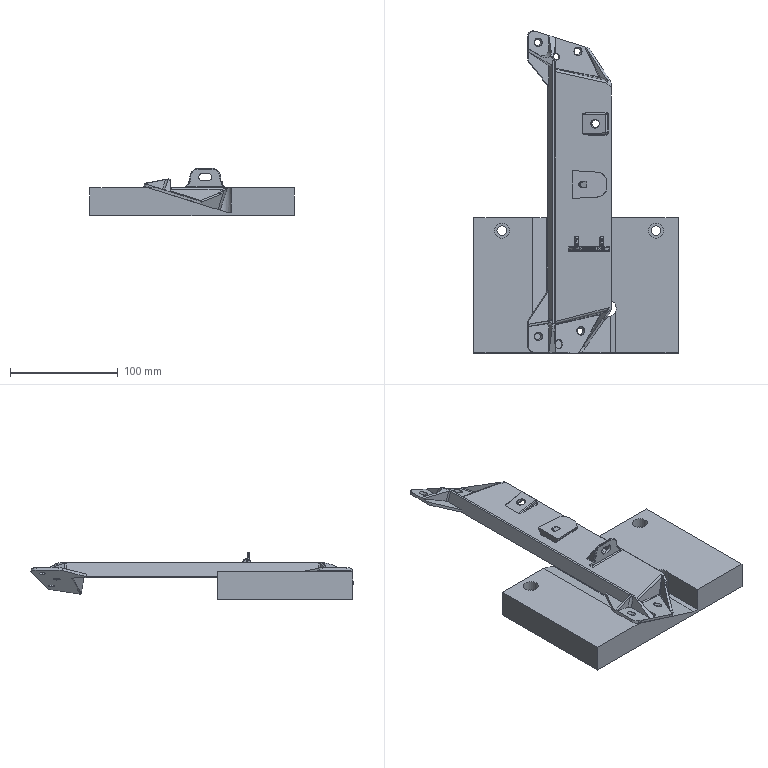NC program | NX | posted with a generic post | part box 190 x 299.709 x 43.804 mm
Whole program:
N10 G17 G21 G94 G90
(PLANAR_MILL_4_COPY_COPY_2_COPY_COPY_1_COPY , TOOL : D4)
N12 T03 M6
N14 G53
N16 G17 G0 G90 X-12.473 Y-11.4 S5800 M3
N18 G43 Z10. H3
N20 Z-95.192
N22 G94 G1 X-9.816 Z-95.206 F2500.
N24 X-9.648 Z-95.207
N26 X-9.199 Y-11.268 Z-95.209
N28 X-8.818 Y-10.997 Z-95.212
N30 X-8.547 Y-10.616 Z-95.214
N32 X-8.416 Y-10.167 Z-95.217
N34 Y-9.832 Z-95.218
N36 X-8.548 Y-9.383 Z-95.221
N38 X-8.819 Y-9.002 Z-95.223
N40 X-9.2 Y-8.731 Z-95.226
N42 X-9.649 Y-8.6 Z-95.228
N44 X-14.987 Z-95.256
N46 X-15.435 Y-8.732 Z-95.258
N48 X-15.816 Y-9.003 Z-95.261
N50 X-16.087 Y-9.384 Z-95.263
N52 X-16.219 Y-9.833 Z-95.266
N54 Y-10.168 Z-95.268
N56 X-16.087 Y-10.617 Z-95.27
N58 X-15.816 Y-10.997 Z-95.272
N60 X-15.435 Y-11.268 Z-95.275
N62 X-14.986 Y-11.4 Z-95.277
N64 X-9.648 Z-95.305
N66 X-9.199 Y-11.268 Z-95.308
N68 X-8.818 Y-10.997 Z-95.31
N70 X-8.547 Y-10.616 Z-95.313
N72 X-8.416 Y-10.167 Z-95.315
N74 Y-9.832 Z-95.317
N76 X-8.548 Y-9.383 Z-95.319
N78 X-8.819 Y-9.002 Z-95.322
N80 X-9.2 Y-8.731 Z-95.324
N82 X-9.649 Y-8.6 Z-95.327
N84 X-14.987 Z-95.355
N86 X-15.435 Y-8.732 Z-95.357
N88 X-15.816 Y-9.003 Z-95.36
N90 X-16.087 Y-9.384 Z-95.362
N92 X-16.219 Y-9.833 Z-95.364
N94 Y-10.168 Z-95.366
N96 X-16.087 Y-10.617 Z-95.369
N98 X-15.816 Y-10.997 Z-95.371
N100 X-15.435 Y-11.268 Z-95.374
N102 X-14.986 Y-11.4 Z-95.376
N104 X-9.648 Z-95.404
N106 X-9.199 Y-11.268 Z-95.406
N108 X-8.818 Y-10.997 Z-95.409
N110 X-8.547 Y-10.616 Z-95.411
N112 X-8.416 Y-10.167 Z-95.414
N114 Y-9.832 Z-95.415
N116 X-8.548 Y-9.383 Z-95.418
N118 X-8.819 Y-9.002 Z-95.42
N120 X-9.2 Y-8.731 Z-95.423
N122 X-9.649 Y-8.6 Z-95.425
N124 X-14.987 Z-95.453
N126 X-15.435 Y-8.732 Z-95.456
N128 X-15.816 Y-9.003 Z-95.458
N130 X-16.087 Y-9.384 Z-95.461
N132 X-16.219 Y-9.833 Z-95.463
N134 Y-10.168 Z-95.465
N136 X-16.087 Y-10.617 Z-95.467
N138 X-15.816 Y-10.997 Z-95.47
N140 X-15.435 Y-11.268 Z-95.472
N142 X-14.986 Y-11.4 Z-95.475
N144 X-9.648 Z-95.502
N146 X-9.199 Y-11.268 Z-95.505
N148 X-8.818 Y-10.997 Z-95.507
N150 X-8.547 Y-10.616 Z-95.51
N152 X-8.416 Y-10.167 Z-95.512
N154 Y-9.832 Z-95.514
N156 X-8.548 Y-9.383 Z-95.516
N158 X-8.819 Y-9.002 Z-95.519
N160 X-9.2 Y-8.731 Z-95.521
N162 X-9.649 Y-8.6 Z-95.524
N164 X-14.987 Z-95.552
N166 X-15.435 Y-8.732 Z-95.554
N168 X-15.816 Y-9.003 Z-95.557
N170 X-16.087 Y-9.384 Z-95.559
N172 X-16.219 Y-9.833 Z-95.562
N174 Y-10.168 Z-95.563
N176 X-16.087 Y-10.617 Z-95.566
N178 X-15.816 Y-10.997 Z-95.568
N180 X-15.435 Y-11.268 Z-95.571
N182 X-14.986 Y-11.4 Z-95.573
N184 X-9.648 Z-95.601
N186 X-9.199 Y-11.268 Z-95.604
N188 X-8.818 Y-10.997 Z-95.606
N190 X-8.547 Y-10.616 Z-95.608
N192 X-8.416 Y-10.167 Z-95.611
N194 Y-9.832 Z-95.613
N196 X-8.548 Y-9.383 Z-95.615
N198 X-8.819 Y-9.002 Z-95.618
N200 X-9.2 Y-8.731 Z-95.62
N202 X-9.649 Y-8.6 Z-95.622
N204 X-14.987 Z-95.65
N206 X-15.435 Y-8.732 Z-95.653
N208 X-15.816 Y-9.003 Z-95.655
N210 X-16.087 Y-9.384 Z-95.658
N212 X-16.219 Y-9.833 Z-95.66
N214 Y-10.168 Z-95.662
N216 X-16.087 Y-10.617 Z-95.664
N218 X-15.816 Y-10.997 Z-95.667
N220 X-15.435 Y-11.268 Z-95.669
N222 X-14.986 Y-11.4 Z-95.672
N224 X-9.648 Z-95.7
N226 X-9.199 Y-11.268 Z-95.702
N228 X-8.818 Y-10.997 Z-95.705
N230 X-8.547 Y-10.616 Z-95.707
N232 X-8.416 Y-10.167 Z-95.709
N234 Y-9.832 Z-95.711
N236 X-8.548 Y-9.383 Z-95.714
N238 X-8.819 Y-9.002 Z-95.716
N240 X-9.2 Y-8.731 Z-95.719
N242 X-9.649 Y-8.6 Z-95.721
N244 X-14.987 Z-95.749
N246 X-15.435 Y-8.732 Z-95.751
N248 X-15.816 Y-9.003 Z-95.754
N250 X-16.087 Y-9.384 Z-95.756
N252 X-16.219 Y-9.833 Z-95.759
N254 Y-10.168 Z-95.76
N256 X-16.087 Y-10.617 Z-95.763
N258 X-15.816 Y-10.997 Z-95.765
N260 X-15.435 Y-11.268 Z-95.768
N262 X-14.986 Y-11.4 Z-95.77
N264 X-9.648 Z-95.798
N266 X-9.199 Y-11.268 Z-95.801
N268 X-8.818 Y-10.997 Z-95.803
N270 X-8.547 Y-10.616 Z-95.806
N272 X-8.416 Y-10.167 Z-95.808
N274 Y-9.832 Z-95.81
N276 X-8.548 Y-9.383 Z-95.812
N278 X-8.819 Y-9.002 Z-95.815
N280 X-9.2 Y-8.731 Z-95.817
N282 X-9.649 Y-8.6 Z-95.82
N284 X-14.987 Z-95.848
N286 X-15.435 Y-8.732 Z-95.85
N288 X-15.816 Y-9.003 Z-95.852
N290 X-16.087 Y-9.384 Z-95.855
N292 X-16.219 Y-9.833 Z-95.857
N294 Y-10.168 Z-95.859
N296 X-16.087 Y-10.617 Z-95.862
N298 X-15.816 Y-10.997 Z-95.864
N300 X-15.435 Y-11.268 Z-95.866
N302 X-14.986 Y-11.4 Z-95.869
N304 X-9.648 Z-95.897
N306 X-9.199 Y-11.268 Z-95.899
N308 X-8.818 Y-10.997 Z-95.902
N310 X-8.547 Y-10.616 Z-95.904
N312 X-8.416 Y-10.167 Z-95.907
N314 Y-9.832 Z-95.908
N316 X-8.548 Y-9.383 Z-95.911
N318 X-8.819 Y-9.002 Z-95.913
N320 X-9.2 Y-8.731 Z-95.916
N322 X-9.649 Y-8.6 Z-95.918
N324 X-14.987 Z-95.946
N326 X-15.435 Y-8.732 Z-95.949
N328 X-15.816 Y-9.003 Z-95.951
N330 X-16.087 Y-9.384 Z-95.953
N332 X-16.219 Y-9.833 Z-95.956
N334 Y-10.168 Z-95.958
N336 X-16.087 Y-10.617 Z-95.96
N338 X-15.816 Y-10.997 Z-95.963
N340 X-15.435 Y-11.268 Z-95.965
N342 X-14.986 Y-11.4 Z-95.967
N344 X-9.648 Z-95.995
N346 X-9.199 Y-11.268 Z-95.998
N348 X-8.818 Y-10.997 Z-96.
N350 X-8.547 Y-10.616 Z-96.003
N352 X-8.416 Y-10.167 Z-96.005
N354 Y-9.832 Z-96.007
N356 X-8.548 Y-9.383 Z-96.009
N358 X-8.819 Y-9.002 Z-96.012
N360 X-9.2 Y-8.731 Z-96.014
N362 X-9.649 Y-8.6 Z-96.017
N364 X-14.987 Z-96.045
N366 X-15.435 Y-8.732 Z-96.047
N368 X-15.816 Y-9.003 Z-96.05
N370 X-16.087 Y-9.384 Z-96.052
N372 X-16.219 Y-9.833 Z-96.054
N374 Y-10.168 Z-96.056
N376 X-16.087 Y-10.617 Z-96.059
N378 X-15.816 Y-10.997 Z-96.061
N380 X-15.435 Y-11.268 Z-96.064
N382 X-14.986 Y-11.4 Z-96.066
N384 X-9.648 Z-96.094
N386 X-9.199 Y-11.268 Z-96.096
N388 X-8.818 Y-10.997 Z-96.099
N390 X-8.547 Y-10.616 Z-96.101
N392 X-8.416 Y-10.167 Z-96.104
N394 Y-9.832 Z-96.106
N396 X-8.548 Y-9.383 Z-96.108
N398 X-8.819 Y-9.002 Z-96.11
N400 X-9.2 Y-8.731 Z-96.113
N402 X-9.649 Y-8.6 Z-96.115
N404 X-14.987 Z-96.143
N406 X-15.435 Y-8.732 Z-96.146
N408 X-15.816 Y-9.003 Z-96.148
N410 X-16.087 Y-9.384 Z-96.151
N412 X-16.219 Y-9.833 Z-96.153
N414 Y-10.168 Z-96.155
N416 X-16.087 Y-10.617 Z-96.157
N418 X-15.816 Y-10.997 Z-96.16
N420 X-15.435 Y-11.268 Z-96.162
N422 X-14.986 Y-11.4 Z-96.165
N424 X-9.648 Z-96.193
N426 X-9.199 Y-11.268 Z-96.195
N428 X-8.818 Y-10.997 Z-96.197
N430 X-8.547 Y-10.616 Z-96.2
N432 X-8.416 Y-10.167 Z-96.202
N434 Y-9.832 Z-96.204
N436 X-8.548 Y-9.383 Z-96.207
N438 X-8.819 Y-9.002 Z-96.209
N440 X-9.2 Y-8.731 Z-96.211
N442 X-9.649 Y-8.6 Z-96.214
N444 X-14.987 Z-96.242
N446 X-15.435 Y-8.732 Z-96.244
N448 X-15.816 Y-9.003 Z-96.247
N450 X-16.087 Y-9.384 Z-96.249
N452 X-16.219 Y-9.833 Z-96.252
N454 Y-10.168 Z-96.253
N456 X-16.087 Y-10.617 Z-96.256
N458 X-15.816 Y-10.997 Z-96.258
N460 X-15.435 Y-11.268 Z-96.261
N462 X-14.986 Y-11.4 Z-96.263
N464 X-9.648 Z-96.291
N466 X-9.199 Y-11.268 Z-96.294
N468 X-8.818 Y-10.997 Z-96.296
N470 X-8.547 Y-10.616 Z-96.299
N472 X-8.416 Y-10.167 Z-96.301
N474 Y-9.832 Z-96.303
N476 X-8.548 Y-9.383 Z-96.305
N478 X-8.819 Y-9.002 Z-96.308
N480 X-9.2 Y-8.731 Z-96.31
N482 X-9.649 Y-8.6 Z-96.312
N484 X-14.987 Z-96.34
N486 X-15.435 Y-8.732 Z-96.343
N488 X-15.816 Y-9.003 Z-96.345
N490 X-16.087 Y-9.384 Z-96.348
N492 X-16.219 Y-9.833 Z-96.35
N494 Y-10.168 Z-96.352
N496 X-16.087 Y-10.617 Z-96.354
N498 X-15.816 Y-10.997 Z-96.357
N500 X-15.435 Y-11.268 Z-96.359
N502 X-14.986 Y-11.4 Z-96.362
N504 X-9.648 Z-96.39
N506 X-9.199 Y-11.268 Z-96.392
N508 X-8.818 Y-10.997 Z-96.395
N510 X-8.547 Y-10.616 Z-96.397
N512 X-8.416 Y-10.167 Z-96.4
N514 Y-9.832 Z-96.401
N516 X-8.548 Y-9.383 Z-96.404
N518 X-8.819 Y-9.002 Z-96.406
N520 X-9.2 Y-8.731 Z-96.409
N522 X-9.649 Y-8.6 Z-96.411
N524 X-14.987 Z-96.439
N526 X-15.435 Y-8.732 Z-96.441
N528 X-15.816 Y-9.003 Z-96.444
N530 X-16.087 Y-9.384 Z-96.446
N532 X-16.219 Y-9.833 Z-96.449
N534 Y-10.168 Z-96.451
N536 X-16.087 Y-10.617 Z-96.453
N538 X-15.816 Y-10.997 Z-96.455
N540 X-15.435 Y-11.268 Z-96.458
N542 X-14.986 Y-11.4 Z-96.46
N544 X-9.648 Z-96.488
N546 X-9.199 Y-11.268 Z-96.491
N548 X-8.818 Y-10.997 Z-96.493
N550 X-8.547 Y-10.616 Z-96.496
N552 X-8.416 Y-10.167 Z-96.498
N554 Y-9.832 Z-96.5
N556 X-8.548 Y-9.383 Z-96.502
N558 X-8.819 Y-9.002 Z-96.505
N560 X-9.2 Y-8.731 Z-96.507
N562 X-9.649 Y-8.6 Z-96.51
N564 X-14.987 Z-96.538
N566 X-15.435 Y-8.732 Z-96.54
N568 X-15.816 Y-9.003 Z-96.543
N570 X-16.087 Y-9.384 Z-96.545
N572 X-16.219 Y-9.833 Z-96.547
N574 Y-10.168 Z-96.549
N576 X-16.087 Y-10.617 Z-96.552
N578 X-15.816 Y-10.997 Z-96.554
N580 X-15.435 Y-11.268 Z-96.557
N582 X-14.986 Y-11.4 Z-96.559
N584 X-9.648 Z-96.587
N586 X-9.199 Y-11.268 Z-96.589
N588 X-8.818 Y-10.997 Z-96.592
N590 X-8.547 Y-10.616 Z-96.594
N592 X-8.416 Y-10.167 Z-96.597
N594 Y-9.832 Z-96.598
N596 X-8.548 Y-9.383 Z-96.601
N598 X-8.819 Y-9.002 Z-96.603
N600 X-9.2 Y-8.731 Z-96.606
N602 X-9.649 Y-8.6 Z-96.608
N604 X-14.987 Z-96.636
N606 X-15.435 Y-8.732 Z-96.639
N608 X-15.816 Y-9.003 Z-96.641
N610 X-16.087 Y-9.384 Z-96.644
N612 X-16.219 Y-9.833 Z-96.646
N614 Y-10.168 Z-96.648
N616 X-16.087 Y-10.617 Z-96.65
N618 X-15.816 Y-10.997 Z-96.653
N620 X-15.435 Y-11.268 Z-96.655
N622 X-14.986 Y-11.4 Z-96.658
N624 X-9.648 Z-96.685
N626 X-9.199 Y-11.268 Z-96.688
N628 X-8.818 Y-10.997 Z-96.69
N630 X-8.547 Y-10.616 Z-96.693
N632 X-8.416 Y-10.167 Z-96.695
N634 Y-9.832 Z-96.697
N636 X-8.548 Y-9.383 Z-96.699
N638 X-8.819 Y-9.002 Z-96.702
N640 X-9.2 Y-8.731 Z-96.704
N642 X-9.649 Y-8.6 Z-96.707
N644 X-14.987 Z-96.735
N646 X-15.435 Y-8.732 Z-96.737
N648 X-15.816 Y-9.003 Z-96.74
N650 X-16.087 Y-9.384 Z-96.742
N652 X-16.219 Y-9.833 Z-96.745
N654 Y-10.168 Z-96.746
N656 X-16.087 Y-10.617 Z-96.749
N658 X-15.816 Y-10.997 Z-96.751
N660 X-15.435 Y-11.268 Z-96.754
N662 X-14.986 Y-11.4 Z-96.756
N664 X-9.648 Z-96.784
N666 X-9.199 Y-11.268 Z-96.787
N668 X-8.818 Y-10.997 Z-96.789
N670 X-8.547 Y-10.616 Z-96.791
N672 X-8.416 Y-10.167 Z-96.794
N674 Y-9.832 Z-96.796
N676 X-8.548 Y-9.383 Z-96.798
N678 X-8.819 Y-9.002 Z-96.801
N680 X-9.2 Y-8.731 Z-96.803
N682 X-9.649 Y-8.6 Z-96.805
N684 X-14.987 Z-96.833
N686 X-15.435 Y-8.732 Z-96.836
N688 X-15.816 Y-9.003 Z-96.838
N690 X-16.087 Y-9.384 Z-96.841
N692 X-16.219 Y-9.833 Z-96.843
N694 Y-10.168 Z-96.845
N696 X-16.087 Y-10.617 Z-96.847
N698 X-15.816 Y-10.997 Z-96.85
N700 X-15.435 Y-11.268 Z-96.852
N702 X-14.986 Y-11.4 Z-96.855
N704 X-9.648 Z-96.883
N706 X-9.199 Y-11.268 Z-96.885
N708 X-8.818 Y-10.997 Z-96.888
N710 X-8.547 Y-10.616 Z-96.89
N712 X-8.416 Y-10.167 Z-96.892
N714 Y-9.832 Z-96.894
N716 X-8.548 Y-9.383 Z-96.897
N718 X-8.819 Y-9.002 Z-96.899
N720 X-9.2 Y-8.731 Z-96.902
N722 X-9.649 Y-8.6 Z-96.904
N724 X-14.987 Z-96.932
N726 X-15.435 Y-8.732 Z-96.934
N728 X-15.816 Y-9.003 Z-96.937
N730 X-16.087 Y-9.384 Z-96.939
N732 X-16.219 Y-9.833 Z-96.942
N734 Y-10.168 Z-96.943
N736 X-16.087 Y-10.617 Z-96.946
N738 X-15.816 Y-10.997 Z-96.948
N740 X-15.435 Y-11.268 Z-96.951
N742 X-14.986 Y-11.4 Z-96.953
N744 X-9.648 Z-96.981
N746 X-9.199 Y-11.268 Z-96.984
N748 X-8.818 Y-10.997 Z-96.986
N750 X-8.547 Y-10.616 Z-96.989
N752 X-8.416 Y-10.167 Z-96.991
N754 Y-9.832 Z-96.993
N756 X-8.548 Y-9.383 Z-96.995
N758 X-8.819 Y-9.002 Z-96.998
N760 X-9.2 Y-8.731 Z-97.
N762 X-9.649 Y-8.6 Z-97.003
N764 X-14.987 Z-97.031
N766 X-15.435 Y-8.732 Z-97.033
N768 X-15.816 Y-9.003 Z-97.035
N770 X-16.087 Y-9.384 Z-97.038
N772 X-16.219 Y-9.833 Z-97.04
N774 Y-10.168 Z-97.042
N776 X-16.087 Y-10.617 Z-97.045
N778 X-15.816 Y-10.997 Z-97.047
N780 X-15.435 Y-11.268 Z-97.049
N782 X-14.986 Y-11.4 Z-97.052
N784 X-9.648 Z-97.08
N786 X-9.199 Y-11.268 Z-97.082
N788 X-8.818 Y-10.997 Z-97.085
N790 X-8.547 Y-10.616 Z-97.087
N792 X-8.416 Y-10.167 Z-97.09
N794 Y-9.832 Z-97.091
N796 X-8.548 Y-9.383 Z-97.094
N798 X-8.819 Y-9.002 Z-97.096
N800 X-9.2 Y-8.731 Z-97.099
N802 X-9.649 Y-8.6 Z-97.101
N804 X-14.987 Z-97.129
N806 X-15.435 Y-8.732 Z-97.132
N808 X-15.816 Y-9.003 Z-97.134
N810 X-16.087 Y-9.384 Z-97.136
N812 X-16.219 Y-9.833 Z-97.139
N814 Y-10.168 Z-97.141
N816 X-16.087 Y-10.617 Z-97.143
N818 X-15.816 Y-10.997 Z-97.146
N820 X-15.435 Y-11.268 Z-97.148
N822 X-14.986 Y-11.4 Z-97.15
N824 X-9.648 Z-97.178
N826 X-9.199 Y-11.268 Z-97.181
N828 X-8.818 Y-10.997 Z-97.183
N830 X-8.547 Y-10.616 Z-97.186
N832 X-8.416 Y-10.167 Z-97.188
N834 Y-9.832 Z-97.19
N836 X-8.548 Y-9.383 Z-97.192
N838 X-8.819 Y-9.002 Z-97.195
N840 X-9.2 Y-8.731 Z-97.197
N842 X-9.649 Y-8.6 Z-97.2
N844 X-14.987 Z-97.228
N846 X-15.435 Y-8.732 Z-97.23
N848 X-15.816 Y-9.003 Z-97.233
N850 X-16.087 Y-9.384 Z-97.235
N852 X-16.219 Y-9.833 Z-97.237
N854 Y-10.168 Z-97.239
N856 X-16.087 Y-10.617 Z-97.242
N858 X-15.816 Y-10.997 Z-97.244
N860 X-15.435 Y-11.268 Z-97.247
N862 X-14.986 Y-11.4 Z-97.249
N864 X-9.648 Z-97.277
N866 X-9.199 Y-11.268 Z-97.279
N868 X-8.818 Y-10.997 Z-97.282
N870 X-8.547 Y-10.616 Z-97.284
N872 X-8.416 Y-10.167 Z-97.287
N874 Y-9.832 Z-97.289
N876 X-8.548 Y-9.383 Z-97.291
N878 X-8.819 Y-9.002 Z-97.293
N880 X-9.2 Y-8.731 Z-97.296
N882 X-9.649 Y-8.6 Z-97.298
N884 X-14.987 Z-97.326
N886 X-15.435 Y-8.732 Z-97.329
N888 X-15.816 Y-9.003 Z-97.331
N890 X-16.087 Y-9.384 Z-97.334
N892 X-16.219 Y-9.833 Z-97.336
N894 Y-10.168 Z-97.338
N896 X-16.087 Y-10.617 Z-97.34
N898 X-15.816 Y-10.997 Z-97.343
N900 X-15.435 Y-11.268 Z-97.345
N902 X-14.986 Y-11.4 Z-97.348
N904 X-9.648 Z-97.376
N906 X-9.199 Y-11.268 Z-97.378
N908 X-8.818 Y-10.997 Z-97.38
N910 X-8.547 Y-10.616 Z-97.383
N912 X-8.416 Y-10.167 Z-97.385
N914 Y-9.832 Z-97.387
N916 X-8.548 Y-9.383 Z-97.39
N918 X-8.819 Y-9.002 Z-97.392
N920 X-9.2 Y-8.731 Z-97.394
N922 X-9.649 Y-8.6 Z-97.397
N924 X-14.987 Z-97.425
N926 X-15.435 Y-8.732 Z-97.427
N928 X-15.816 Y-9.003 Z-97.43
N930 X-16.087 Y-9.384 Z-97.432
N932 X-16.219 Y-9.833 Z-97.435
N934 Y-10.168 Z-97.436
N936 X-16.087 Y-10.617 Z-97.439
N938 X-15.816 Y-10.997 Z-97.441
N940 X-15.435 Y-11.268 Z-97.444
N942 X-14.986 Y-11.4 Z-97.446
N944 X-9.648 Z-97.474
N946 X-9.199 Y-11.268 Z-97.477
N948 X-8.818 Y-10.997 Z-97.479
N950 X-8.547 Y-10.616 Z-97.482
N952 X-8.416 Y-10.167 Z-97.484
N954 Y-9.832 Z-97.486
N956 X-8.548 Y-9.383 Z-97.488
N958 X-8.819 Y-9.002 Z-97.491
N960 X-9.2 Y-8.731 Z-97.493
N962 X-9.649 Y-8.6 Z-97.496
N964 X-14.987 Z-97.523
N966 X-15.435 Y-8.732 Z-97.526
N968 X-15.816 Y-9.003 Z-97.528
N970 X-16.087 Y-9.384 Z-97.531
N972 X-16.219 Y-9.833 Z-97.533
N974 Y-10.168 Z-97.535
N976 X-16.087 Y-10.617 Z-97.537
N978 X-15.816 Y-10.997 Z-97.54
N980 X-15.435 Y-11.268 Z-97.542
N982 X-14.986 Y-11.4 Z-97.545
N984 X-9.648 Z-97.573
N986 X-9.199 Y-11.268 Z-97.575
N988 X-8.818 Y-10.997 Z-97.578
N990 X-8.547 Y-10.616 Z-97.58
N992 X-8.416 Y-10.167 Z-97.583
N994 Y-9.832 Z-97.584
N996 X-8.548 Y-9.383 Z-97.587
N998 X-8.819 Y-9.002 Z-97.589
N1000 X-9.2 Y-8.731 Z-97.592
N1002 X-9.649 Y-8.6 Z-97.594
N1004 X-14.987 Z-97.622
N1006 X-15.435 Y-8.732 Z-97.624
N1008 X-15.816 Y-9.003 Z-97.627
N1010 X-16.087 Y-9.384 Z-97.629
N1012 X-16.219 Y-9.833 Z-97.632
N1014 Y-10.168 Z-97.634
N1016 X-16.087 Y-10.617 Z-97.636
N1018 X-15.816 Y-10.997 Z-97.638
N1020 X-15.435 Y-11.268 Z-97.641
N1022 X-14.986 Y-11.4 Z-97.643
N1024 X-9.648 Z-97.671
N1026 X-9.199 Y-11.268 Z-97.674
N1028 X-8.818 Y-10.997 Z-97.676
N1030 X-8.547 Y-10.616 Z-97.679
N1032 X-8.416 Y-10.167 Z-97.681
N1034 Y-9.832 Z-97.683
N1036 X-8.548 Y-9.383 Z-97.685
N1038 X-8.819 Y-9.002 Z-97.688
N1040 X-9.2 Y-8.731 Z-97.69
N1042 X-9.649 Y-8.6 Z-97.693
N1044 X-14.987 Z-97.721
N1046 X-15.435 Y-8.732 Z-97.723
N1048 X-15.816 Y-9.003 Z-97.726
N1050 X-16.087 Y-9.384 Z-97.728
N1052 X-16.219 Y-9.833 Z-97.73
N1054 Y-10.168 Z-97.732
N1056 X-16.087 Y-10.617 Z-97.735
N1058 X-15.816 Y-10.997 Z-97.737
N1060 X-15.435 Y-11.268 Z-97.74
N1062 X-14.986 Y-11.4 Z-97.742
N1064 X-9.648 Z-97.77
N1066 X-9.199 Y-11.268 Z-97.772
N1068 X-8.818 Y-10.997 Z-97.775
N1070 X-8.547 Y-10.616 Z-97.777
N1072 X-8.416 Y-10.167 Z-97.78
N1074 Y-9.832 Z-97.781
N1076 X-8.548 Y-9.383 Z-97.784
N1078 X-8.819 Y-9.002 Z-97.786
N1080 X-9.2 Y-8.731 Z-97.789
N1082 X-9.649 Y-8.6 Z-97.791
N1084 X-14.987 Z-97.819
N1086 X-15.435 Y-8.732 Z-97.822
N1088 X-15.816 Y-9.003 Z-97.824
N1090 X-16.087 Y-9.384 Z-97.827
N1092 X-16.219 Y-9.833 Z-97.829
N1094 Y-10.168 Z-97.831
N1096 X-16.087 Y-10.617 Z-97.833
N1098 X-15.816 Y-10.997 Z-97.836
N1100 X-15.435 Y-11.268 Z-97.838
N1102 X-14.986 Y-11.4 Z-97.841
N1104 X-9.648 Z-97.868
N1106 X-9.199 Y-11.268 Z-97.871
N1108 X-8.818 Y-10.997 Z-97.873
N1110 X-8.547 Y-10.616 Z-97.876
N1112 X-8.416 Y-10.167 Z-97.878
N1114 Y-9.832 Z-97.88
N1116 X-8.548 Y-9.383 Z-97.882
N1118 X-8.819 Y-9.002 Z-97.885
N1120 X-9.2 Y-8.731 Z-97.887
N1122 X-9.649 Y-8.6 Z-97.89
N1124 X-14.987 Z-97.918
N1126 X-15.435 Y-8.732 Z-97.92
N1128 X-15.816 Y-9.003 Z-97.923
N1130 X-16.087 Y-9.384 Z-97.925
N1132 X-16.219 Y-9.833 Z-97.928
N1134 Y-10.168 Z-97.929
N1136 X-16.087 Y-10.617 Z-97.932
N1138 X-15.816 Y-10.997 Z-97.934
N1140 X-15.435 Y-11.268 Z-97.937
N1142 X-14.986 Y-11.4 Z-97.939
N1144 X-9.648 Z-97.967
N1146 X-9.199 Y-11.268 Z-97.97
N1148 X-8.818 Y-10.997 Z-97.972
N1150 X-8.547 Y-10.616 Z-97.974
N1152 X-8.416 Y-10.167 Z-97.977
N1154 Y-9.832 Z-97.979
N1156 X-8.548 Y-9.383 Z-97.981
N1158 X-8.819 Y-9.002 Z-97.984
N1160 X-9.2 Y-8.731 Z-97.986
N1162 X-9.649 Y-8.6 Z-97.988
N1164 X-14.987 Z-98.016
N1166 X-15.435 Y-8.732 Z-98.019
N1168 X-15.816 Y-9.003 Z-98.021
N1170 X-16.087 Y-9.384 Z-98.024
N1172 X-16.219 Y-9.833 Z-98.026
N1174 Y-10.168 Z-98.028
N1176 X-16.087 Y-10.617 Z-98.03
N1178 X-15.816 Y-10.997 Z-98.033
N1180 X-15.435 Y-11.268 Z-98.035
N1182 X-14.986 Y-11.4 Z-98.038
N1184 X-9.648 Z-98.066
N1186 X-9.199 Y-11.268 Z-98.068
N1188 X-8.818 Y-10.997 Z-98.071
N1190 X-8.547 Y-10.616 Z-98.073
N1192 X-8.416 Y-10.167 Z-98.075
N1194 Y-9.832 Z-98.077
N1196 X-8.548 Y-9.383 Z-98.08
N1198 X-8.819 Y-9.002 Z-98.082
N1200 X-9.2 Y-8.731 Z-98.085
N1202 X-9.649 Y-8.6 Z-98.087
N1204 X-14.987 Z-98.115
N1206 X-15.435 Y-8.732 Z-98.117
N1208 X-15.816 Y-9.003 Z-98.12
N1210 X-16.087 Y-9.384 Z-98.122
N1212 X-16.219 Y-9.833 Z-98.125
N1214 Y-10.168 Z-98.127
N1216 X-16.087 Y-10.617 Z-98.129
N1218 X-15.816 Y-10.997 Z-98.131
N1220 X-15.435 Y-11.268 Z-98.134
N1222 X-14.986 Y-11.4 Z-98.136
N1224 X-9.648 Z-98.164
N1226 X-9.199 Y-11.268 Z-98.167
N1228 X-8.818 Y-10.997 Z-98.169
N1230 X-8.547 Y-10.616 Z-98.172
N1232 X-8.416 Y-10.167 Z-98.174
N1234 Y-9.832 Z-98.176
N1236 X-8.548 Y-9.383 Z-98.178
N1238 X-8.819 Y-9.002 Z-98.181
N1240 X-9.2 Y-8.731 Z-98.183
N1242 X-9.649 Y-8.6 Z-98.186
N1244 X-14.987 Z-98.214
N1246 X-15.435 Y-8.732 Z-98.216
N1248 X-15.816 Y-9.003 Z-98.218
N1250 X-16.087 Y-9.384 Z-98.221
N1252 X-16.219 Y-9.833 Z-98.223
N1254 Y-10.168 Z-98.225
N1256 X-16.087 Y-10.617 Z-98.228
N1258 X-15.816 Y-10.997 Z-98.23
N1260 X-15.435 Y-11.268 Z-98.232
N1262 X-14.986 Y-11.4 Z-98.235
N1264 X-9.648 Z-98.263
N1266 X-9.199 Y-11.268 Z-98.265
N1268 X-8.818 Y-10.997 Z-98.268
N1270 X-8.547 Y-10.616 Z-98.27
N1272 X-8.416 Y-10.167 Z-98.273
N1274 Y-9.832 Z-98.274
N1276 X-8.548 Y-9.383 Z-98.277
N1278 X-8.819 Y-9.002 Z-98.279
N1280 X-9.2 Y-8.731 Z-98.282
N1282 X-9.649 Y-8.6 Z-98.284
N1284 X-14.987 Z-98.312
N1286 X-15.435 Y-8.732 Z-98.315
N1288 X-15.816 Y-9.003 Z-98.317
N1290 X-16.087 Y-9.384 Z-98.319
N1292 X-16.219 Y-9.833 Z-98.322
N1294 Y-10.168 Z-98.324
N1296 X-16.087 Y-10.617 Z-98.326
N1298 X-15.816 Y-10.997 Z-98.329
N1300 X-15.435 Y-11.268 Z-98.331
N1302 X-14.986 Y-11.4 Z-98.333
N1304 X-9.648 Z-98.361
N1306 X-9.199 Y-11.268 Z-98.364
N1308 X-8.818 Y-10.997 Z-98.366
N1310 X-8.547 Y-10.616 Z-98.369
N1312 X-8.416 Y-10.167 Z-98.371
N1314 Y-9.832 Z-98.373
N1316 X-8.548 Y-9.383 Z-98.375
N1318 X-8.819 Y-9.002 Z-98.378
N1320 X-9.2 Y-8.731 Z-98.38
N1322 X-9.649 Y-8.6 Z-98.383
N1324 X-9.817 Z-98.384
N1326 X-14.819
N1328 G3 X-16.219 Y-10. R1.4
N1330 X-14.818 Y-11.4 R1.4
N1332 G1 X-9.816
N1334 G3 X-8.416 Y-10. R1.4
N1336 X-9.817 Y-8.6 R1.4
N1338 G1 Z-98.084
N1340 G0 Z10.
(PLANAR_MILL_4_COPY_COPY_2_COPY_COPY_1_COPY_COPY , TOOL : D4)
N1342 X-8.816 Y-9.499
N1344 Z-97.884
N1346 G1 Z-98.384 F800.
N1348 G3 X-9.817 Y-8.5 R1.
N1350 G1 X-14.819
N1352 G3 X-16.319 Y-10. R1.5
N1354 X-14.818 Y-11.5 R1.5
N1356 G1 X-9.816
N1358 G3 X-8.316 Y-10. R1.5
N1360 X-9.817 Y-8.5 R1.5
N1362 X-10.816 Y-9.501 R1.
N1364 G1 Z-97.884
N1366 G0 Z10.
N1368 M5
N1370 M2